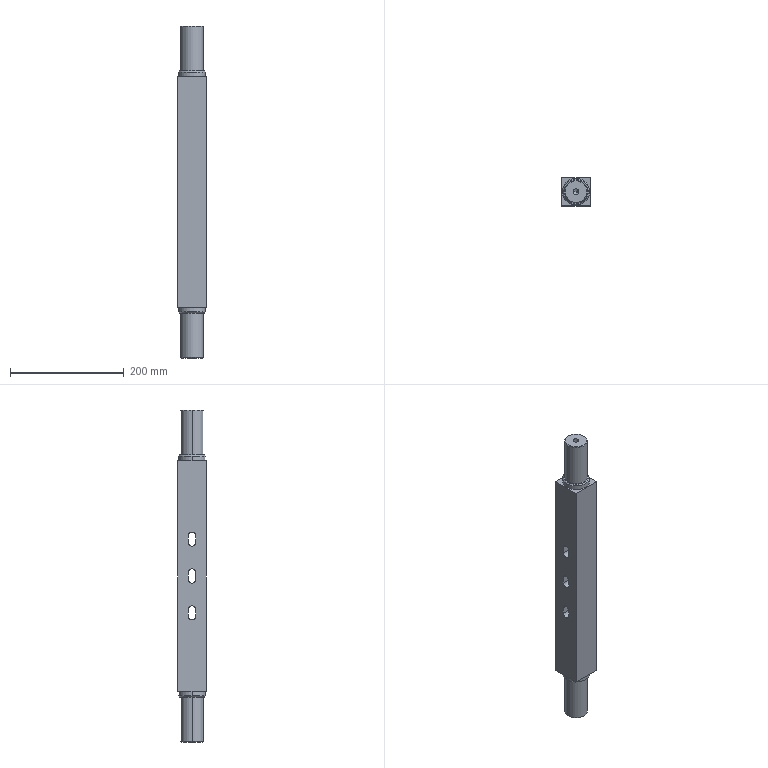Part | SolidWorks | features ICE 5, Chamfer 3, HoleWzd 2, Extrusion 1 | 1 solid | 46 faces | box 50 x 50 x 584.5 mm | volume 1201279 mm3 | cylinder 18 | plane 16 | cone 12 | commonest cylinder face diameters 13 x6 10.2 x4 40 x4 47.5 x4
STEP:
#1=CARTESIAN_POINT('',(-5.1,0.,555.25));
#2=VERTEX_POINT('',#1);
#3=CARTESIAN_POINT('',(5.1,0.,555.25));
#4=VERTEX_POINT('',#3);
#5=CARTESIAN_POINT('',(0.,0.,555.25));
#6=DIRECTION('',(0.,0.,1.));
#7=DIRECTION('',(1.,0.,0.));
#8=AXIS2_PLACEMENT_3D('',#5,#6,#7);
#9=CIRCLE('',#8,5.1);
#10=EDGE_CURVE('',#2,#4,#9,.T.);
#11=ORIENTED_EDGE('',*,*,#10,.F.);
#12=CARTESIAN_POINT('',(-5.1,0.,584.5));
#13=VERTEX_POINT('',#12);
#14=CARTESIAN_POINT('',(-5.1,0.,584.5));
#15=DIRECTION('',(0.,0.,1.));
#16=VECTOR('',#15,1000.);
#17=LINE('',#14,#16);
#18=EDGE_CURVE('',#2,#13,#17,.T.);
#19=ORIENTED_EDGE('',*,*,#18,.T.);
#20=CARTESIAN_POINT('',(5.1,0.,584.5));
#21=VERTEX_POINT('',#20);
#22=CARTESIAN_POINT('',(0.,0.,584.5));
#23=DIRECTION('',(0.,0.,1.));
#24=DIRECTION('',(1.,0.,0.));
#25=AXIS2_PLACEMENT_3D('',#22,#23,#24);
#26=CIRCLE('',#25,5.1);
#27=EDGE_CURVE('',#13,#21,#26,.T.);
#28=ORIENTED_EDGE('',*,*,#27,.T.);
#29=CARTESIAN_POINT('',(5.1,0.,584.5));
#30=DIRECTION('',(0.,0.,1.));
#31=VECTOR('',#30,1000.);
#32=LINE('',#29,#31);
#33=EDGE_CURVE('',#4,#21,#32,.T.);
#34=ORIENTED_EDGE('',*,*,#33,.F.);
#35=EDGE_LOOP('',(#11,#19,#28,#34));
#36=FACE_OUTER_BOUND('',#35,.T.);
#37=CARTESIAN_POINT('',(0.,0.,584.5));
#38=DIRECTION('',(0.,0.,1.));
#39=DIRECTION('',(1.,0.,0.));
#40=AXIS2_PLACEMENT_3D('',#37,#38,#39);
#41=CYLINDRICAL_SURFACE('',#40,5.1);
#42=ADVANCED_FACE('',(#36),#41,.F.);
#43=CARTESIAN_POINT('',(0.,0.,552.186));
#44=VERTEX_POINT('',#43);
#45=CARTESIAN_POINT('',(5.1,0.,555.25));
#46=DIRECTION('',(0.8572,0.,0.515));
#47=VECTOR('',#46,1000.);
#48=LINE('',#45,#47);
#49=EDGE_CURVE('',#44,#4,#48,.T.);
#50=ORIENTED_EDGE('',*,*,#49,.F.);
#51=CARTESIAN_POINT('',(-5.1,0.,555.25));
#52=DIRECTION('',(-0.8572,0.,0.515));
#53=VECTOR('',#52,1000.);
#54=LINE('',#51,#53);
#55=EDGE_CURVE('',#44,#2,#54,.T.);
#56=ORIENTED_EDGE('',*,*,#55,.T.);
#57=ORIENTED_EDGE('',*,*,#10,.T.);
#58=EDGE_LOOP('',(#50,#56,#57));
#59=FACE_OUTER_BOUND('',#58,.T.);
#60=CARTESIAN_POINT('',(0.,0.,555.25));
#61=DIRECTION('',(0.,0.,1.));
#62=DIRECTION('',(1.,0.,0.));
#63=AXIS2_PLACEMENT_3D('',#60,#61,#62);
#64=CONICAL_SURFACE('',#63,5.1,1.03);
#65=ADVANCED_FACE('',(#59),#64,.F.);
#66=CARTESIAN_POINT('',(5.1,0.,29.25));
#67=VERTEX_POINT('',#66);
#68=CARTESIAN_POINT('',(-5.1,0.,29.25));
#69=VERTEX_POINT('',#68);
#70=CARTESIAN_POINT('',(0.,0.,29.25));
#71=DIRECTION('',(0.,0.,-1.));
#72=DIRECTION('',(-1.,0.,0.));
#73=AXIS2_PLACEMENT_3D('',#70,#71,#72);
#74=CIRCLE('',#73,5.1);
#75=EDGE_CURVE('',#67,#69,#74,.T.);
#76=ORIENTED_EDGE('',*,*,#75,.F.);
#77=CARTESIAN_POINT('',(5.1,0.,0.));
#78=VERTEX_POINT('',#77);
#79=CARTESIAN_POINT('',(5.1,0.,0.));
#80=DIRECTION('',(0.,0.,-1.));
#81=VECTOR('',#80,1000.);
#82=LINE('',#79,#81);
#83=EDGE_CURVE('',#67,#78,#82,.T.);
#84=ORIENTED_EDGE('',*,*,#83,.T.);
#85=CARTESIAN_POINT('',(-5.1,0.,0.));
#86=VERTEX_POINT('',#85);
#87=CARTESIAN_POINT('',(0.,0.,0.));
#88=DIRECTION('',(0.,0.,-1.));
#89=DIRECTION('',(-1.,0.,0.));
#90=AXIS2_PLACEMENT_3D('',#87,#88,#89);
#91=CIRCLE('',#90,5.1);
#92=EDGE_CURVE('',#78,#86,#91,.T.);
#93=ORIENTED_EDGE('',*,*,#92,.T.);
#94=CARTESIAN_POINT('',(-5.1,0.,0.));
#95=DIRECTION('',(0.,0.,-1.));
#96=VECTOR('',#95,1000.);
#97=LINE('',#94,#96);
#98=EDGE_CURVE('',#69,#86,#97,.T.);
#99=ORIENTED_EDGE('',*,*,#98,.F.);
#100=EDGE_LOOP('',(#76,#84,#93,#99));
#101=FACE_OUTER_BOUND('',#100,.T.);
#102=CARTESIAN_POINT('',(0.,0.,0.));
#103=DIRECTION('',(0.,0.,-1.));
#104=DIRECTION('',(-1.,0.,0.));
#105=AXIS2_PLACEMENT_3D('',#102,#103,#104);
#106=CYLINDRICAL_SURFACE('',#105,5.1);
#107=ADVANCED_FACE('',(#101),#106,.F.);
#108=CARTESIAN_POINT('',(0.,0.,32.314));
#109=VERTEX_POINT('',#108);
#110=CARTESIAN_POINT('',(-5.1,0.,29.25));
#111=DIRECTION('',(-0.8572,0.,-0.515));
#112=VECTOR('',#111,1000.);
#113=LINE('',#110,#112);
#114=EDGE_CURVE('',#109,#69,#113,.T.);
#115=ORIENTED_EDGE('',*,*,#114,.F.);
#116=CARTESIAN_POINT('',(5.1,0.,29.25));
#117=DIRECTION('',(0.8572,0.,-0.515));
#118=VECTOR('',#117,1000.);
#119=LINE('',#116,#118);
#120=EDGE_CURVE('',#109,#67,#119,.T.);
#121=ORIENTED_EDGE('',*,*,#120,.T.);
#122=ORIENTED_EDGE('',*,*,#75,.T.);
#123=EDGE_LOOP('',(#115,#121,#122));
#124=FACE_OUTER_BOUND('',#123,.T.);
#125=CARTESIAN_POINT('',(0.,0.,29.25));
#126=DIRECTION('',(0.,0.,-1.));
#127=DIRECTION('',(-1.,0.,0.));
#128=AXIS2_PLACEMENT_3D('',#125,#126,#127);
#129=CONICAL_SURFACE('',#128,5.1,1.03);
#130=ADVANCED_FACE('',(#124),#129,.F.);
#131=CARTESIAN_POINT('',(19.,0.,584.5));
#132=VERTEX_POINT('',#131);
#133=CARTESIAN_POINT('',(-19.,0.,584.5));
#134=VERTEX_POINT('',#133);
#135=CARTESIAN_POINT('',(0.,0.,584.5));
#136=DIRECTION('',(0.,0.,1.));
#137=DIRECTION('',(1.,0.,0.));
#138=AXIS2_PLACEMENT_3D('',#135,#136,#137);
#139=CIRCLE('',#138,19.);
#140=EDGE_CURVE('',#132,#134,#139,.T.);
#141=ORIENTED_EDGE('',*,*,#140,.F.);
#142=CARTESIAN_POINT('',(20.,0.,583.5));
#143=VERTEX_POINT('',#142);
#144=CARTESIAN_POINT('',(19.,0.,584.5));
#145=DIRECTION('',(0.7071,0.,-0.7071));
#146=VECTOR('',#145,1000.);
#147=LINE('',#144,#146);
#148=EDGE_CURVE('',#132,#143,#147,.T.);
#149=ORIENTED_EDGE('',*,*,#148,.T.);
#150=CARTESIAN_POINT('',(-20.,0.,583.5));
#151=VERTEX_POINT('',#150);
#152=CARTESIAN_POINT('',(0.,0.,583.5));
#153=DIRECTION('',(0.,0.,-1.));
#154=DIRECTION('',(1.,0.,0.));
#155=AXIS2_PLACEMENT_3D('',#152,#153,#154);
#156=CIRCLE('',#155,20.);
#157=EDGE_CURVE('',#151,#143,#156,.T.);
#158=ORIENTED_EDGE('',*,*,#157,.F.);
#159=CARTESIAN_POINT('',(-19.,0.,584.5));
#160=DIRECTION('',(-0.7071,0.,-0.7071));
#161=VECTOR('',#160,1000.);
#162=LINE('',#159,#161);
#163=EDGE_CURVE('',#134,#151,#162,.T.);
#164=ORIENTED_EDGE('',*,*,#163,.F.);
#165=EDGE_LOOP('',(#141,#149,#158,#164));
#166=FACE_OUTER_BOUND('',#165,.T.);
#167=CARTESIAN_POINT('',(0.,0.,584.5));
#168=DIRECTION('',(0.,0.,-1.));
#169=DIRECTION('',(-1.,0.,0.));
#170=AXIS2_PLACEMENT_3D('',#167,#168,#169);
#171=CONICAL_SURFACE('',#170,19.,0.7854);
#172=ADVANCED_FACE('',(#166),#171,.T.);
#173=CARTESIAN_POINT('',(-19.,0.,0.));
#174=VERTEX_POINT('',#173);
#175=CARTESIAN_POINT('',(19.,0.,0.));
#176=VERTEX_POINT('',#175);
#177=CARTESIAN_POINT('',(0.,0.,0.));
#178=DIRECTION('',(0.,0.,-1.));
#179=DIRECTION('',(1.,0.,0.));
#180=AXIS2_PLACEMENT_3D('',#177,#178,#179);
#181=CIRCLE('',#180,19.);
#182=EDGE_CURVE('',#174,#176,#181,.T.);
#183=ORIENTED_EDGE('',*,*,#182,.F.);
#184=CARTESIAN_POINT('',(-20.,0.,1.));
#185=VERTEX_POINT('',#184);
#186=CARTESIAN_POINT('',(-20.,0.,1.));
#187=DIRECTION('',(-0.7071,0.,0.7071));
#188=VECTOR('',#187,1000.);
#189=LINE('',#186,#188);
#190=EDGE_CURVE('',#174,#185,#189,.T.);
#191=ORIENTED_EDGE('',*,*,#190,.T.);
#192=CARTESIAN_POINT('',(20.,0.,1.));
#193=VERTEX_POINT('',#192);
#194=CARTESIAN_POINT('',(0.,0.,1.));
#195=DIRECTION('',(0.,0.,1.));
#196=DIRECTION('',(1.,0.,0.));
#197=AXIS2_PLACEMENT_3D('',#194,#195,#196);
#198=CIRCLE('',#197,20.);
#199=EDGE_CURVE('',#193,#185,#198,.T.);
#200=ORIENTED_EDGE('',*,*,#199,.F.);
#201=CARTESIAN_POINT('',(20.,0.,1.));
#202=DIRECTION('',(0.7071,0.,0.7071));
#203=VECTOR('',#202,1000.);
#204=LINE('',#201,#203);
#205=EDGE_CURVE('',#176,#193,#204,.T.);
#206=ORIENTED_EDGE('',*,*,#205,.F.);
#207=EDGE_LOOP('',(#183,#191,#200,#206));
#208=FACE_OUTER_BOUND('',#207,.T.);
#209=CARTESIAN_POINT('',(0.,0.,1.));
#210=DIRECTION('',(0.,0.,1.));
#211=DIRECTION('',(1.,0.,0.));
#212=AXIS2_PLACEMENT_3D('',#209,#210,#211);
#213=CONICAL_SURFACE('',#212,20.,0.7854);
#214=ADVANCED_FACE('',(#208),#213,.T.);
#215=ORIENTED_EDGE('',*,*,#157,.T.);
#216=CARTESIAN_POINT('',(20.,0.,505.5));
#217=VERTEX_POINT('',#216);
#218=CARTESIAN_POINT('',(20.,0.,584.5));
#219=DIRECTION('',(0.,0.,-1.));
#220=VECTOR('',#219,1000.);
#221=LINE('',#218,#220);
#222=EDGE_CURVE('',#143,#217,#221,.T.);
#223=ORIENTED_EDGE('',*,*,#222,.T.);
#224=CARTESIAN_POINT('',(-20.,0.,505.5));
#225=VERTEX_POINT('',#224);
#226=CARTESIAN_POINT('',(0.,0.,505.5));
#227=DIRECTION('',(0.,0.,1.));
#228=DIRECTION('',(1.,0.,0.));
#229=AXIS2_PLACEMENT_3D('',#226,#227,#228);
#230=CIRCLE('',#229,20.);
#231=EDGE_CURVE('',#217,#225,#230,.T.);
#232=ORIENTED_EDGE('',*,*,#231,.T.);
#233=CARTESIAN_POINT('',(-20.,0.,584.5));
#234=DIRECTION('',(0.,0.,-1.));
#235=VECTOR('',#234,1000.);
#236=LINE('',#233,#235);
#237=EDGE_CURVE('',#151,#225,#236,.T.);
#238=ORIENTED_EDGE('',*,*,#237,.F.);
#239=EDGE_LOOP('',(#215,#223,#232,#238));
#240=FACE_OUTER_BOUND('',#239,.T.);
#241=CARTESIAN_POINT('',(0.,0.,584.5));
#242=DIRECTION('',(0.,0.,-1.));
#243=DIRECTION('',(-1.,0.,0.));
#244=AXIS2_PLACEMENT_3D('',#241,#242,#243);
#245=CYLINDRICAL_SURFACE('',#244,20.);
#246=ADVANCED_FACE('',(#240),#245,.T.);
#247=CARTESIAN_POINT('',(21.75,0.,505.5));
#248=VERTEX_POINT('',#247);
#249=CARTESIAN_POINT('',(-21.75,0.,505.5));
#250=VERTEX_POINT('',#249);
#251=CARTESIAN_POINT('',(0.,0.,505.5));
#252=DIRECTION('',(0.,0.,1.));
#253=DIRECTION('',(1.,0.,0.));
#254=AXIS2_PLACEMENT_3D('',#251,#252,#253);
#255=CIRCLE('',#254,21.75);
#256=EDGE_CURVE('',#248,#250,#255,.T.);
#257=ORIENTED_EDGE('',*,*,#256,.F.);
#258=CARTESIAN_POINT('',(23.75,0.,503.5));
#259=VERTEX_POINT('',#258);
#260=CARTESIAN_POINT('',(21.75,0.,505.5));
#261=DIRECTION('',(0.7071,0.,-0.7071));
#262=VECTOR('',#261,1000.);
#263=LINE('',#260,#262);
#264=EDGE_CURVE('',#248,#259,#263,.T.);
#265=ORIENTED_EDGE('',*,*,#264,.T.);
#266=CARTESIAN_POINT('',(-23.75,0.,503.5));
#267=VERTEX_POINT('',#266);
#268=CARTESIAN_POINT('',(0.,0.,503.5));
#269=DIRECTION('',(0.,0.,-1.));
#270=DIRECTION('',(1.,0.,0.));
#271=AXIS2_PLACEMENT_3D('',#268,#269,#270);
#272=CIRCLE('',#271,23.75);
#273=EDGE_CURVE('',#267,#259,#272,.T.);
#274=ORIENTED_EDGE('',*,*,#273,.F.);
#275=CARTESIAN_POINT('',(-21.75,0.,505.5));
#276=DIRECTION('',(-0.7071,0.,-0.7071));
#277=VECTOR('',#276,1000.);
#278=LINE('',#275,#277);
#279=EDGE_CURVE('',#250,#267,#278,.T.);
#280=ORIENTED_EDGE('',*,*,#279,.F.);
#281=EDGE_LOOP('',(#257,#265,#274,#280));
#282=FACE_OUTER_BOUND('',#281,.T.);
#283=CARTESIAN_POINT('',(0.,0.,505.5));
#284=DIRECTION('',(0.,0.,-1.));
#285=DIRECTION('',(-1.,0.,0.));
#286=AXIS2_PLACEMENT_3D('',#283,#284,#285);
#287=CONICAL_SURFACE('',#286,21.75,0.7854);
#288=ADVANCED_FACE('',(#282),#287,.T.);
#289=ORIENTED_EDGE('',*,*,#273,.T.);
#290=CARTESIAN_POINT('',(23.75,0.,495.5));
#291=VERTEX_POINT('',#290);
#292=CARTESIAN_POINT('',(23.75,0.,505.5));
#293=DIRECTION('',(0.,0.,-1.));
#294=VECTOR('',#293,1000.);
#295=LINE('',#292,#294);
#296=EDGE_CURVE('',#259,#291,#295,.T.);
#297=ORIENTED_EDGE('',*,*,#296,.T.);
#298=CARTESIAN_POINT('',(-23.75,0.,495.5));
#299=VERTEX_POINT('',#298);
#300=CARTESIAN_POINT('',(0.,0.,495.5));
#301=DIRECTION('',(0.,0.,1.));
#302=DIRECTION('',(1.,0.,0.));
#303=AXIS2_PLACEMENT_3D('',#300,#301,#302);
#304=CIRCLE('',#303,23.75);
#305=EDGE_CURVE('',#291,#299,#304,.T.);
#306=ORIENTED_EDGE('',*,*,#305,.T.);
#307=CARTESIAN_POINT('',(-23.75,0.,505.5));
#308=DIRECTION('',(0.,0.,-1.));
#309=VECTOR('',#308,1000.);
#310=LINE('',#307,#309);
#311=EDGE_CURVE('',#267,#299,#310,.T.);
#312=ORIENTED_EDGE('',*,*,#311,.F.);
#313=EDGE_LOOP('',(#289,#297,#306,#312));
#314=FACE_OUTER_BOUND('',#313,.T.);
#315=CARTESIAN_POINT('',(0.,0.,505.5));
#316=DIRECTION('',(0.,0.,-1.));
#317=DIRECTION('',(-1.,0.,0.));
#318=AXIS2_PLACEMENT_3D('',#315,#316,#317);
#319=CYLINDRICAL_SURFACE('',#318,23.75);
#320=ADVANCED_FACE('',(#314),#319,.T.);
#321=CARTESIAN_POINT('',(-21.75,0.,79.));
#322=VERTEX_POINT('',#321);
#323=CARTESIAN_POINT('',(21.75,0.,79.));
#324=VERTEX_POINT('',#323);
#325=CARTESIAN_POINT('',(0.,0.,79.));
#326=DIRECTION('',(0.,0.,-1.));
#327=DIRECTION('',(1.,0.,0.));
#328=AXIS2_PLACEMENT_3D('',#325,#326,#327);
#329=CIRCLE('',#328,21.75);
#330=EDGE_CURVE('',#322,#324,#329,.T.);
#331=ORIENTED_EDGE('',*,*,#330,.F.);
#332=CARTESIAN_POINT('',(-23.75,0.,81.));
#333=VERTEX_POINT('',#332);
#334=CARTESIAN_POINT('',(-23.75,0.,81.));
#335=DIRECTION('',(-0.7071,0.,0.7071));
#336=VECTOR('',#335,1000.);
#337=LINE('',#334,#336);
#338=EDGE_CURVE('',#322,#333,#337,.T.);
#339=ORIENTED_EDGE('',*,*,#338,.T.);
#340=CARTESIAN_POINT('',(23.75,0.,81.));
#341=VERTEX_POINT('',#340);
#342=CARTESIAN_POINT('',(0.,0.,81.));
#343=DIRECTION('',(0.,0.,1.));
#344=DIRECTION('',(1.,0.,0.));
#345=AXIS2_PLACEMENT_3D('',#342,#343,#344);
#346=CIRCLE('',#345,23.75);
#347=EDGE_CURVE('',#341,#333,#346,.T.);
#348=ORIENTED_EDGE('',*,*,#347,.F.);
#349=CARTESIAN_POINT('',(23.75,0.,81.));
#350=DIRECTION('',(0.7071,0.,0.7071));
#351=VECTOR('',#350,1000.);
#352=LINE('',#349,#351);
#353=EDGE_CURVE('',#324,#341,#352,.T.);
#354=ORIENTED_EDGE('',*,*,#353,.F.);
#355=EDGE_LOOP('',(#331,#339,#348,#354));
#356=FACE_OUTER_BOUND('',#355,.T.);
#357=CARTESIAN_POINT('',(0.,0.,81.));
#358=DIRECTION('',(0.,0.,1.));
#359=DIRECTION('',(1.,0.,0.));
#360=AXIS2_PLACEMENT_3D('',#357,#358,#359);
#361=CONICAL_SURFACE('',#360,23.75,0.7854);
#362=ADVANCED_FACE('',(#356),#361,.T.);
#363=CARTESIAN_POINT('',(23.75,0.,89.));
#364=VERTEX_POINT('',#363);
#365=CARTESIAN_POINT('',(-23.75,0.,89.));
#366=VERTEX_POINT('',#365);
#367=CARTESIAN_POINT('',(0.,0.,89.));
#368=DIRECTION('',(0.,0.,1.));
#369=DIRECTION('',(1.,0.,0.));
#370=AXIS2_PLACEMENT_3D('',#367,#368,#369);
#371=CIRCLE('',#370,23.75);
#372=EDGE_CURVE('',#364,#366,#371,.T.);
#373=ORIENTED_EDGE('',*,*,#372,.F.);
#374=CARTESIAN_POINT('',(23.75,0.,89.));
#375=DIRECTION('',(0.,0.,-1.));
#376=VECTOR('',#375,1000.);
#377=LINE('',#374,#376);
#378=EDGE_CURVE('',#364,#341,#377,.T.);
#379=ORIENTED_EDGE('',*,*,#378,.T.);
#380=ORIENTED_EDGE('',*,*,#347,.T.);
#381=CARTESIAN_POINT('',(-23.75,0.,89.));
#382=DIRECTION('',(0.,0.,-1.));
#383=VECTOR('',#382,1000.);
#384=LINE('',#381,#383);
#385=EDGE_CURVE('',#366,#333,#384,.T.);
#386=ORIENTED_EDGE('',*,*,#385,.F.);
#387=EDGE_LOOP('',(#373,#379,#380,#386));
#388=FACE_OUTER_BOUND('',#387,.T.);
#389=CARTESIAN_POINT('',(0.,0.,89.));
#390=DIRECTION('',(0.,0.,-1.));
#391=DIRECTION('',(-1.,0.,0.));
#392=AXIS2_PLACEMENT_3D('',#389,#390,#391);
#393=CYLINDRICAL_SURFACE('',#392,23.75);
#394=ADVANCED_FACE('',(#388),#393,.T.);
#395=CARTESIAN_POINT('',(20.,0.,79.));
#396=VERTEX_POINT('',#395);
#397=CARTESIAN_POINT('',(-20.,0.,79.));
#398=VERTEX_POINT('',#397);
#399=CARTESIAN_POINT('',(0.,0.,79.));
#400=DIRECTION('',(0.,0.,1.));
#401=DIRECTION('',(1.,0.,0.));
#402=AXIS2_PLACEMENT_3D('',#399,#400,#401);
#403=CIRCLE('',#402,20.);
#404=EDGE_CURVE('',#396,#398,#403,.T.);
#405=ORIENTED_EDGE('',*,*,#404,.F.);
#406=CARTESIAN_POINT('',(20.,0.,79.));
#407=DIRECTION('',(0.,0.,-1.));
#408=VECTOR('',#407,1000.);
#409=LINE('',#406,#408);
#410=EDGE_CURVE('',#396,#193,#409,.T.);
#411=ORIENTED_EDGE('',*,*,#410,.T.);
#412=ORIENTED_EDGE('',*,*,#199,.T.);
#413=CARTESIAN_POINT('',(-20.,0.,79.));
#414=DIRECTION('',(0.,0.,-1.));
#415=VECTOR('',#414,1000.);
#416=LINE('',#413,#415);
#417=EDGE_CURVE('',#398,#185,#416,.T.);
#418=ORIENTED_EDGE('',*,*,#417,.F.);
#419=EDGE_LOOP('',(#405,#411,#412,#418));
#420=FACE_OUTER_BOUND('',#419,.T.);
#421=CARTESIAN_POINT('',(0.,0.,79.));
#422=DIRECTION('',(0.,0.,-1.));
#423=DIRECTION('',(-1.,0.,0.));
#424=AXIS2_PLACEMENT_3D('',#421,#422,#423);
#425=CYLINDRICAL_SURFACE('',#424,20.);
#426=ADVANCED_FACE('',(#420),#425,.T.);
#427=ORIENTED_EDGE('',*,*,#410,.F.);
#428=CARTESIAN_POINT('',(0.,0.,79.));
#429=DIRECTION('',(0.,0.,1.));
#430=DIRECTION('',(1.,0.,0.));
#431=AXIS2_PLACEMENT_3D('',#428,#429,#430);
#432=CIRCLE('',#431,20.);
#433=EDGE_CURVE('',#398,#396,#432,.T.);
#434=ORIENTED_EDGE('',*,*,#433,.F.);
#435=ORIENTED_EDGE('',*,*,#417,.T.);
#436=CARTESIAN_POINT('',(0.,0.,1.));
#437=DIRECTION('',(0.,0.,1.));
#438=DIRECTION('',(1.,0.,0.));
#439=AXIS2_PLACEMENT_3D('',#436,#437,#438);
#440=CIRCLE('',#439,20.);
#441=EDGE_CURVE('',#185,#193,#440,.T.);
#442=ORIENTED_EDGE('',*,*,#441,.T.);
#443=EDGE_LOOP('',(#427,#434,#435,#442));
#444=FACE_OUTER_BOUND('',#443,.T.);
#445=CARTESIAN_POINT('',(0.,0.,79.));
#446=DIRECTION('',(0.,0.,-1.));
#447=DIRECTION('',(-1.,0.,0.));
#448=AXIS2_PLACEMENT_3D('',#445,#446,#447);
#449=CYLINDRICAL_SURFACE('',#448,20.);
#450=ADVANCED_FACE('',(#444),#449,.T.);
#451=CARTESIAN_POINT('',(0.,0.,0.));
#452=DIRECTION('',(0.,0.,-1.));
#453=DIRECTION('',(-1.,0.,0.));
#454=AXIS2_PLACEMENT_3D('',#451,#452,#453);
#455=CIRCLE('',#454,5.1);
#456=EDGE_CURVE('',#86,#78,#455,.T.);
#457=ORIENTED_EDGE('',*,*,#456,.F.);
#458=ORIENTED_EDGE('',*,*,#92,.F.);
#459=EDGE_LOOP('',(#457,#458));
#460=FACE_BOUND('',#459,.T.);
#461=CARTESIAN_POINT('',(0.,0.,0.));
#462=DIRECTION('',(0.,0.,-1.));
#463=DIRECTION('',(1.,0.,0.));
#464=AXIS2_PLACEMENT_3D('',#461,#462,#463);
#465=CIRCLE('',#464,19.);
#466=EDGE_CURVE('',#176,#174,#465,.T.);
#467=ORIENTED_EDGE('',*,*,#466,.T.);
#468=ORIENTED_EDGE('',*,*,#182,.T.);
#469=EDGE_LOOP('',(#467,#468));
#470=FACE_OUTER_BOUND('',#469,.T.);
#471=CARTESIAN_POINT('',(0.,0.,0.));
#472=DIRECTION('',(0.,0.,1.));
#473=DIRECTION('',(1.,0.,0.));
#474=AXIS2_PLACEMENT_3D('',#471,#472,#473);
#475=PLANE('',#474);
#476=ADVANCED_FACE('',(#460,#470),#475,.F.);
#477=ORIENTED_EDGE('',*,*,#378,.F.);
#478=CARTESIAN_POINT('',(0.,0.,89.));
#479=DIRECTION('',(0.,0.,1.));
#480=DIRECTION('',(1.,0.,0.));
#481=AXIS2_PLACEMENT_3D('',#478,#479,#480);
#482=CIRCLE('',#481,23.75);
#483=EDGE_CURVE('',#366,#364,#482,.T.);
#484=ORIENTED_EDGE('',*,*,#483,.F.);
#485=ORIENTED_EDGE('',*,*,#385,.T.);
#486=CARTESIAN_POINT('',(0.,0.,81.));
#487=DIRECTION('',(0.,0.,1.));
#488=DIRECTION('',(1.,0.,0.));
#489=AXIS2_PLACEMENT_3D('',#486,#487,#488);
#490=CIRCLE('',#489,23.75);
#491=EDGE_CURVE('',#333,#341,#490,.T.);
#492=ORIENTED_EDGE('',*,*,#491,.T.);
#493=EDGE_LOOP('',(#477,#484,#485,#492));
#494=FACE_OUTER_BOUND('',#493,.T.);
#495=CARTESIAN_POINT('',(0.,0.,89.));
#496=DIRECTION('',(0.,0.,-1.));
#497=DIRECTION('',(-1.,0.,0.));
#498=AXIS2_PLACEMENT_3D('',#495,#496,#497);
#499=CYLINDRICAL_SURFACE('',#498,23.75);
#500=ADVANCED_FACE('',(#494),#499,.T.);
#501=CARTESIAN_POINT('',(0.,0.,79.));
#502=DIRECTION('',(0.,0.,-1.));
#503=DIRECTION('',(1.,0.,0.));
#504=AXIS2_PLACEMENT_3D('',#501,#502,#503);
#505=CIRCLE('',#504,21.75);
#506=EDGE_CURVE('',#324,#322,#505,.T.);
#507=ORIENTED_EDGE('',*,*,#506,.T.);
#508=ORIENTED_EDGE('',*,*,#330,.T.);
#509=EDGE_LOOP('',(#507,#508));
#510=FACE_OUTER_BOUND('',#509,.T.);
#511=ORIENTED_EDGE('',*,*,#433,.T.);
#512=ORIENTED_EDGE('',*,*,#404,.T.);
#513=EDGE_LOOP('',(#511,#512));
#514=FACE_BOUND('',#513,.T.);
#515=CARTESIAN_POINT('',(0.,0.,79.));
#516=DIRECTION('',(0.,0.,1.));
#517=DIRECTION('',(1.,0.,0.));
#518=AXIS2_PLACEMENT_3D('',#515,#516,#517);
#519=PLANE('',#518);
#520=ADVANCED_FACE('',(#510,#514),#519,.F.);
#521=ORIENTED_EDGE('',*,*,#338,.F.);
#522=ORIENTED_EDGE('',*,*,#506,.F.);
#523=ORIENTED_EDGE('',*,*,#353,.T.);
#524=ORIENTED_EDGE('',*,*,#491,.F.);
#525=EDGE_LOOP('',(#521,#522,#523,#524));
#526=FACE_OUTER_BOUND('',#525,.T.);
#527=CARTESIAN_POINT('',(0.,0.,81.));
#528=DIRECTION('',(0.,0.,1.));
#529=DIRECTION('',(1.,0.,0.));
#530=AXIS2_PLACEMENT_3D('',#527,#528,#529);
#531=CONICAL_SURFACE('',#530,23.75,0.7854);
#532=ADVANCED_FACE('',(#526),#531,.T.);
#533=CARTESIAN_POINT('',(-25.,6.5,351.25));
#534=VERTEX_POINT('',#533);
#535=CARTESIAN_POINT('',(-25.,6.5,363.25));
#536=VERTEX_POINT('',#535);
#537=CARTESIAN_POINT('',(-25.,6.5,495.5));
#538=DIRECTION('',(0.,0.,1.));
#539=VECTOR('',#538,1000.);
#540=LINE('',#537,#539);
#541=EDGE_CURVE('',#534,#536,#540,.T.);
#542=ORIENTED_EDGE('',*,*,#541,.T.);
#543=CARTESIAN_POINT('',(-25.,-6.5,363.25));
#544=VERTEX_POINT('',#543);
#545=CARTESIAN_POINT('',(-25.,0.,363.25));
#546=DIRECTION('',(1.,0.,0.));
#547=DIRECTION('',(0.,1.,0.));
#548=AXIS2_PLACEMENT_3D('',#545,#546,#547);
#549=CIRCLE('',#548,6.5);
#550=EDGE_CURVE('',#536,#544,#549,.T.);
#551=ORIENTED_EDGE('',*,*,#550,.T.);
#552=CARTESIAN_POINT('',(-25.,-6.5,351.25));
#553=VERTEX_POINT('',#552);
#554=CARTESIAN_POINT('',(-25.,-6.5,495.5));
#555=DIRECTION('',(0.,0.,-1.));
#556=VECTOR('',#555,1000.);
#557=LINE('',#554,#556);
#558=EDGE_CURVE('',#544,#553,#557,.T.);
#559=ORIENTED_EDGE('',*,*,#558,.T.);
#560=CARTESIAN_POINT('',(-25.,0.,351.25));
#561=DIRECTION('',(1.,0.,0.));
#562=DIRECTION('',(0.,1.,0.));
#563=AXIS2_PLACEMENT_3D('',#560,#561,#562);
#564=CIRCLE('',#563,6.5);
#565=EDGE_CURVE('',#553,#534,#564,.T.);
#566=ORIENTED_EDGE('',*,*,#565,.T.);
#567=EDGE_LOOP('',(#542,#551,#559,#566));
#568=FACE_BOUND('',#567,.T.);
#569=CARTESIAN_POINT('',(-25.,6.5,286.25));
#570=VERTEX_POINT('',#569);
#571=CARTESIAN_POINT('',(-25.,6.5,298.25));
#572=VERTEX_POINT('',#571);
#573=CARTESIAN_POINT('',(-25.,6.5,495.5));
#574=DIRECTION('',(0.,0.,1.));
#575=VECTOR('',#574,1000.);
#576=LINE('',#573,#575);
#577=EDGE_CURVE('',#570,#572,#576,.T.);
#578=ORIENTED_EDGE('',*,*,#577,.T.);
#579=CARTESIAN_POINT('',(-25.,-6.5,298.25));
#580=VERTEX_POINT('',#579);
#581=CARTESIAN_POINT('',(-25.,0.,298.25));
#582=DIRECTION('',(1.,0.,0.));
#583=DIRECTION('',(0.,1.,0.));
#584=AXIS2_PLACEMENT_3D('',#581,#582,#583);
#585=CIRCLE('',#584,6.5);
#586=EDGE_CURVE('',#572,#580,#585,.T.);
#587=ORIENTED_EDGE('',*,*,#586,.T.);
#588=CARTESIAN_POINT('',(-25.,-6.5,286.25));
#589=VERTEX_POINT('',#588);
#590=CARTESIAN_POINT('',(-25.,-6.5,495.5));
#591=DIRECTION('',(0.,0.,-1.));
#592=VECTOR('',#591,1000.);
#593=LINE('',#590,#592);
#594=EDGE_CURVE('',#580,#589,#593,.T.);
#595=ORIENTED_EDGE('',*,*,#594,.T.);
#596=CARTESIAN_POINT('',(-25.,0.,286.25));
#597=DIRECTION('',(1.,0.,0.));
#598=DIRECTION('',(0.,1.,0.));
#599=AXIS2_PLACEMENT_3D('',#596,#597,#598);
#600=CIRCLE('',#599,6.5);
#601=EDGE_CURVE('',#589,#570,#600,.T.);
#602=ORIENTED_EDGE('',*,*,#601,.T.);
#603=EDGE_LOOP('',(#578,#587,#595,#602));
#604=FACE_BOUND('',#603,.T.);
#605=CARTESIAN_POINT('',(-25.,6.5,221.25));
#606=VERTEX_POINT('',#605);
#607=CARTESIAN_POINT('',(-25.,6.5,233.25));
#608=VERTEX_POINT('',#607);
#609=CARTESIAN_POINT('',(-25.,6.5,495.5));
#610=DIRECTION('',(0.,0.,1.));
#611=VECTOR('',#610,1000.);
#612=LINE('',#609,#611);
#613=EDGE_CURVE('',#606,#608,#612,.T.);
#614=ORIENTED_EDGE('',*,*,#613,.T.);
#615=CARTESIAN_POINT('',(-25.,-6.5,233.25));
#616=VERTEX_POINT('',#615);
#617=CARTESIAN_POINT('',(-25.,0.,233.25));
#618=DIRECTION('',(1.,0.,0.));
#619=DIRECTION('',(0.,1.,0.));
#620=AXIS2_PLACEMENT_3D('',#617,#618,#619);
#621=CIRCLE('',#620,6.5);
#622=EDGE_CURVE('',#608,#616,#621,.T.);
#623=ORIENTED_EDGE('',*,*,#622,.T.);
#624=CARTESIAN_POINT('',(-25.,-6.5,221.25));
#625=VERTEX_POINT('',#624);
#626=CARTESIAN_POINT('',(-25.,-6.5,495.5));
#627=DIRECTION('',(0.,0.,-1.));
#628=VECTOR('',#627,1000.);
#629=LINE('',#626,#628);
#630=EDGE_CURVE('',#616,#625,#629,.T.);
#631=ORIENTED_EDGE('',*,*,#630,.T.);
#632=CARTESIAN_POINT('',(-25.,0.,221.25));
#633=DIRECTION('',(1.,0.,0.));
#634=DIRECTION('',(0.,1.,0.));
#635=AXIS2_PLACEMENT_3D('',#632,#633,#634);
#636=CIRCLE('',#635,6.5);
#637=EDGE_CURVE('',#625,#606,#636,.T.);
#638=ORIENTED_EDGE('',*,*,#637,.T.);
#639=EDGE_LOOP('',(#614,#623,#631,#638));
#640=FACE_BOUND('',#639,.T.);
#641=CARTESIAN_POINT('',(-25.,25.,89.));
#642=VERTEX_POINT('',#641);
#643=CARTESIAN_POINT('',(-25.,-25.,89.));
#644=VERTEX_POINT('',#643);
#645=CARTESIAN_POINT('',(-25.,25.,89.));
#646=DIRECTION('',(0.,-1.,0.));
#647=VECTOR('',#646,1000.);
#648=LINE('',#645,#647);
#649=EDGE_CURVE('',#642,#644,#648,.T.);
#650=ORIENTED_EDGE('',*,*,#649,.T.);
#651=CARTESIAN_POINT('',(-25.,-25.,495.5));
#652=VERTEX_POINT('',#651);
#653=CARTESIAN_POINT('',(-25.,-25.,495.5));
#654=DIRECTION('',(0.,0.,-1.));
#655=VECTOR('',#654,1000.);
#656=LINE('',#653,#655);
#657=EDGE_CURVE('',#652,#644,#656,.T.);
#658=ORIENTED_EDGE('',*,*,#657,.F.);
#659=CARTESIAN_POINT('',(-25.,25.,495.5));
#660=VERTEX_POINT('',#659);
#661=CARTESIAN_POINT('',(-25.,25.,495.5));
#662=DIRECTION('',(0.,-1.,0.));
#663=VECTOR('',#662,1000.);
#664=LINE('',#661,#663);
#665=EDGE_CURVE('',#660,#652,#664,.T.);
#666=ORIENTED_EDGE('',*,*,#665,.F.);
#667=CARTESIAN_POINT('',(-25.,25.,495.5));
#668=DIRECTION('',(0.,0.,-1.));
#669=VECTOR('',#668,1000.);
#670=LINE('',#667,#669);
#671=EDGE_CURVE('',#660,#642,#670,.T.);
#672=ORIENTED_EDGE('',*,*,#671,.T.);
#673=EDGE_LOOP('',(#650,#658,#666,#672));
#674=FACE_OUTER_BOUND('',#673,.T.);
#675=CARTESIAN_POINT('',(-25.,25.,495.5));
#676=DIRECTION('',(1.,0.,0.));
#677=DIRECTION('',(0.,1.,0.));
#678=AXIS2_PLACEMENT_3D('',#675,#676,#677);
#679=PLANE('',#678);
#680=ADVANCED_FACE('',(#568,#604,#640,#674),#679,.F.);
#681=CARTESIAN_POINT('',(25.,-25.,89.));
#682=VERTEX_POINT('',#681);
#683=CARTESIAN_POINT('',(25.,-25.,89.));
#684=DIRECTION('',(1.,0.,0.));
#685=VECTOR('',#684,1000.);
#686=LINE('',#683,#685);
#687=EDGE_CURVE('',#644,#682,#686,.T.);
#688=ORIENTED_EDGE('',*,*,#687,.T.);
#689=CARTESIAN_POINT('',(25.,-25.,495.5));
#690=VERTEX_POINT('',#689);
#691=CARTESIAN_POINT('',(25.,-25.,495.5));
#692=DIRECTION('',(0.,0.,-1.));
#693=VECTOR('',#692,1000.);
#694=LINE('',#691,#693);
#695=EDGE_CURVE('',#690,#682,#694,.T.);
#696=ORIENTED_EDGE('',*,*,#695,.F.);
#697=CARTESIAN_POINT('',(25.,-25.,495.5));
#698=DIRECTION('',(1.,0.,0.));
#699=VECTOR('',#698,1000.);
#700=LINE('',#697,#699);
#701=EDGE_CURVE('',#652,#690,#700,.T.);
#702=ORIENTED_EDGE('',*,*,#701,.F.);
#703=ORIENTED_EDGE('',*,*,#657,.T.);
#704=EDGE_LOOP('',(#688,#696,#702,#703));
#705=FACE_OUTER_BOUND('',#704,.T.);
#706=CARTESIAN_POINT('',(25.,-25.,495.5));
#707=DIRECTION('',(0.,1.,0.));
#708=DIRECTION('',(-1.,0.,0.));
#709=AXIS2_PLACEMENT_3D('',#706,#707,#708);
#710=PLANE('',#709);
#711=ADVANCED_FACE('',(#705),#710,.F.);
#712=CARTESIAN_POINT('',(25.,-6.5,363.25));
#713=VERTEX_POINT('',#712);
#714=CARTESIAN_POINT('',(25.,-6.5,351.25));
#715=VERTEX_POINT('',#714);
#716=CARTESIAN_POINT('',(25.,-6.5,363.25));
#717=DIRECTION('',(0.,0.,-1.));
#718=VECTOR('',#717,1000.);
#719=LINE('',#716,#718);
#720=EDGE_CURVE('',#713,#715,#719,.T.);
#721=ORIENTED_EDGE('',*,*,#720,.F.);
#722=CARTESIAN_POINT('',(25.,6.5,363.25));
#723=VERTEX_POINT('',#722);
#724=CARTESIAN_POINT('',(25.,0.,363.25));
#725=DIRECTION('',(1.,0.,0.));
#726=DIRECTION('',(0.,1.,0.));
#727=AXIS2_PLACEMENT_3D('',#724,#725,#726);
#728=CIRCLE('',#727,6.5);
#729=EDGE_CURVE('',#723,#713,#728,.T.);
#730=ORIENTED_EDGE('',*,*,#729,.F.);
#731=CARTESIAN_POINT('',(25.,6.5,351.25));
#732=VERTEX_POINT('',#731);
#733=CARTESIAN_POINT('',(25.,6.5,363.25));
#734=DIRECTION('',(0.,0.,1.));
#735=VECTOR('',#734,1000.);
#736=LINE('',#733,#735);
#737=EDGE_CURVE('',#732,#723,#736,.T.);
#738=ORIENTED_EDGE('',*,*,#737,.F.);
#739=CARTESIAN_POINT('',(25.,0.,351.25));
#740=DIRECTION('',(1.,0.,0.));
#741=DIRECTION('',(0.,1.,0.));
#742=AXIS2_PLACEMENT_3D('',#739,#740,#741);
#743=CIRCLE('',#742,6.5);
#744=EDGE_CURVE('',#715,#732,#743,.T.);
#745=ORIENTED_EDGE('',*,*,#744,.F.);
#746=EDGE_LOOP('',(#721,#730,#738,#745));
#747=FACE_BOUND('',#746,.T.);
#748=CARTESIAN_POINT('',(25.,-6.5,298.25));
#749=VERTEX_POINT('',#748);
#750=CARTESIAN_POINT('',(25.,-6.5,286.25));
#751=VERTEX_POINT('',#750);
#752=CARTESIAN_POINT('',(25.,-6.5,298.25));
#753=DIRECTION('',(0.,0.,-1.));
#754=VECTOR('',#753,1000.);
#755=LINE('',#752,#754);
#756=EDGE_CURVE('',#749,#751,#755,.T.);
#757=ORIENTED_EDGE('',*,*,#756,.F.);
#758=CARTESIAN_POINT('',(25.,6.5,298.25));
#759=VERTEX_POINT('',#758);
#760=CARTESIAN_POINT('',(25.,0.,298.25));
#761=DIRECTION('',(1.,0.,0.));
#762=DIRECTION('',(0.,1.,0.));
#763=AXIS2_PLACEMENT_3D('',#760,#761,#762);
#764=CIRCLE('',#763,6.5);
#765=EDGE_CURVE('',#759,#749,#764,.T.);
#766=ORIENTED_EDGE('',*,*,#765,.F.);
#767=CARTESIAN_POINT('',(25.,6.5,286.25));
#768=VERTEX_POINT('',#767);
#769=CARTESIAN_POINT('',(25.,6.5,298.25));
#770=DIRECTION('',(0.,0.,1.));
#771=VECTOR('',#770,1000.);
#772=LINE('',#769,#771);
#773=EDGE_CURVE('',#768,#759,#772,.T.);
#774=ORIENTED_EDGE('',*,*,#773,.F.);
#775=CARTESIAN_POINT('',(25.,0.,286.25));
#776=DIRECTION('',(1.,0.,0.));
#777=DIRECTION('',(0.,1.,0.));
#778=AXIS2_PLACEMENT_3D('',#775,#776,#777);
#779=CIRCLE('',#778,6.5);
#780=EDGE_CURVE('',#751,#768,#779,.T.);
#781=ORIENTED_EDGE('',*,*,#780,.F.);
#782=EDGE_LOOP('',(#757,#766,#774,#781));
#783=FACE_BOUND('',#782,.T.);
#784=CARTESIAN_POINT('',(25.,-6.5,233.25));
#785=VERTEX_POINT('',#784);
#786=CARTESIAN_POINT('',(25.,-6.5,221.25));
#787=VERTEX_POINT('',#786);
#788=CARTESIAN_POINT('',(25.,-6.5,233.25));
#789=DIRECTION('',(0.,0.,-1.));
#790=VECTOR('',#789,1000.);
#791=LINE('',#788,#790);
#792=EDGE_CURVE('',#785,#787,#791,.T.);
#793=ORIENTED_EDGE('',*,*,#792,.F.);
#794=CARTESIAN_POINT('',(25.,6.5,233.25));
#795=VERTEX_POINT('',#794);
#796=CARTESIAN_POINT('',(25.,0.,233.25));
#797=DIRECTION('',(1.,0.,0.));
#798=DIRECTION('',(0.,1.,0.));
#799=AXIS2_PLACEMENT_3D('',#796,#797,#798);
#800=CIRCLE('',#799,6.5);
#801=EDGE_CURVE('',#795,#785,#800,.T.);
#802=ORIENTED_EDGE('',*,*,#801,.F.);
#803=CARTESIAN_POINT('',(25.,6.5,221.25));
#804=VERTEX_POINT('',#803);
#805=CARTESIAN_POINT('',(25.,6.5,233.25));
#806=DIRECTION('',(0.,0.,1.));
#807=VECTOR('',#806,1000.);
#808=LINE('',#805,#807);
#809=EDGE_CURVE('',#804,#795,#808,.T.);
#810=ORIENTED_EDGE('',*,*,#809,.F.);
#811=CARTESIAN_POINT('',(25.,0.,221.25));
#812=DIRECTION('',(1.,0.,0.));
#813=DIRECTION('',(0.,1.,0.));
#814=AXIS2_PLACEMENT_3D('',#811,#812,#813);
#815=CIRCLE('',#814,6.5);
#816=EDGE_CURVE('',#787,#804,#815,.T.);
#817=ORIENTED_EDGE('',*,*,#816,.F.);
#818=EDGE_LOOP('',(#793,#802,#810,#817));
#819=FACE_BOUND('',#818,.T.);
#820=CARTESIAN_POINT('',(25.,25.,89.));
#821=VERTEX_POINT('',#820);
#822=CARTESIAN_POINT('',(25.,25.,89.));
#823=DIRECTION('',(0.,1.,0.));
#824=VECTOR('',#823,1000.);
#825=LINE('',#822,#824);
#826=EDGE_CURVE('',#682,#821,#825,.T.);
#827=ORIENTED_EDGE('',*,*,#826,.T.);
#828=CARTESIAN_POINT('',(25.,25.,495.5));
#829=VERTEX_POINT('',#828);
#830=CARTESIAN_POINT('',(25.,25.,495.5));
#831=DIRECTION('',(0.,0.,-1.));
#832=VECTOR('',#831,1000.);
#833=LINE('',#830,#832);
#834=EDGE_CURVE('',#829,#821,#833,.T.);
#835=ORIENTED_EDGE('',*,*,#834,.F.);
#836=CARTESIAN_POINT('',(25.,25.,495.5));
#837=DIRECTION('',(0.,1.,0.));
#838=VECTOR('',#837,1000.);
#839=LINE('',#836,#838);
#840=EDGE_CURVE('',#690,#829,#839,.T.);
#841=ORIENTED_EDGE('',*,*,#840,.F.);
#842=ORIENTED_EDGE('',*,*,#695,.T.);
#843=EDGE_LOOP('',(#827,#835,#841,#842));
#844=FACE_OUTER_BOUND('',#843,.T.);
#845=CARTESIAN_POINT('',(25.,25.,495.5));
#846=DIRECTION('',(-1.,0.,0.));
#847=DIRECTION('',(0.,-1.,0.));
#848=AXIS2_PLACEMENT_3D('',#845,#846,#847);
#849=PLANE('',#848);
#850=ADVANCED_FACE('',(#747,#783,#819,#844),#849,.F.);
#851=CARTESIAN_POINT('',(25.,25.,89.));
#852=DIRECTION('',(-1.,0.,0.));
#853=VECTOR('',#852,1000.);
#854=LINE('',#851,#853);
#855=EDGE_CURVE('',#821,#642,#854,.T.);
#856=ORIENTED_EDGE('',*,*,#855,.T.);
#857=ORIENTED_EDGE('',*,*,#671,.F.);
#858=CARTESIAN_POINT('',(25.,25.,495.5));
#859=DIRECTION('',(-1.,0.,0.));
#860=VECTOR('',#859,1000.);
#861=LINE('',#858,#860);
#862=EDGE_CURVE('',#829,#660,#861,.T.);
#863=ORIENTED_EDGE('',*,*,#862,.F.);
#864=ORIENTED_EDGE('',*,*,#834,.T.);
#865=EDGE_LOOP('',(#856,#857,#863,#864));
#866=FACE_OUTER_BOUND('',#865,.T.);
#867=CARTESIAN_POINT('',(25.,25.,495.5));
#868=DIRECTION('',(0.,-1.,0.));
#869=DIRECTION('',(1.,0.,0.));
#870=AXIS2_PLACEMENT_3D('',#867,#868,#869);
#871=PLANE('',#870);
#872=ADVANCED_FACE('',(#866),#871,.F.);
#873=CARTESIAN_POINT('',(0.,0.,495.5));
#874=DIRECTION('',(0.,0.,1.));
#875=DIRECTION('',(1.,0.,0.));
#876=AXIS2_PLACEMENT_3D('',#873,#874,#875);
#877=CIRCLE('',#876,23.75);
#878=EDGE_CURVE('',#299,#291,#877,.T.);
#879=ORIENTED_EDGE('',*,*,#878,.F.);
#880=ORIENTED_EDGE('',*,*,#305,.F.);
#881=EDGE_LOOP('',(#879,#880));
#882=FACE_BOUND('',#881,.T.);
#883=ORIENTED_EDGE('',*,*,#665,.T.);
#884=ORIENTED_EDGE('',*,*,#701,.T.);
#885=ORIENTED_EDGE('',*,*,#840,.T.);
#886=ORIENTED_EDGE('',*,*,#862,.T.);
#887=EDGE_LOOP('',(#883,#884,#885,#886));
#888=FACE_OUTER_BOUND('',#887,.T.);
#889=CARTESIAN_POINT('',(0.,0.,495.5));
#890=DIRECTION('',(0.,0.,-1.));
#891=DIRECTION('',(-1.,0.,0.));
#892=AXIS2_PLACEMENT_3D('',#889,#890,#891);
#893=PLANE('',#892);
#894=ADVANCED_FACE('',(#882,#888),#893,.F.);
#895=ORIENTED_EDGE('',*,*,#483,.T.);
#896=ORIENTED_EDGE('',*,*,#372,.T.);
#897=EDGE_LOOP('',(#895,#896));
#898=FACE_BOUND('',#897,.T.);
#899=ORIENTED_EDGE('',*,*,#649,.F.);
#900=ORIENTED_EDGE('',*,*,#855,.F.);
#901=ORIENTED_EDGE('',*,*,#826,.F.);
#902=ORIENTED_EDGE('',*,*,#687,.F.);
#903=EDGE_LOOP('',(#899,#900,#901,#902));
#904=FACE_OUTER_BOUND('',#903,.T.);
#905=CARTESIAN_POINT('',(0.,0.,89.));
#906=DIRECTION('',(0.,0.,-1.));
#907=DIRECTION('',(-1.,0.,0.));
#908=AXIS2_PLACEMENT_3D('',#905,#906,#907);
#909=PLANE('',#908);
#910=ADVANCED_FACE('',(#898,#904),#909,.T.);
#911=ORIENTED_EDGE('',*,*,#296,.F.);
#912=CARTESIAN_POINT('',(0.,0.,503.5));
#913=DIRECTION('',(0.,0.,-1.));
#914=DIRECTION('',(1.,0.,0.));
#915=AXIS2_PLACEMENT_3D('',#912,#913,#914);
#916=CIRCLE('',#915,23.75);
#917=EDGE_CURVE('',#259,#267,#916,.T.);
#918=ORIENTED_EDGE('',*,*,#917,.T.);
#919=ORIENTED_EDGE('',*,*,#311,.T.);
#920=ORIENTED_EDGE('',*,*,#878,.T.);
#921=EDGE_LOOP('',(#911,#918,#919,#920));
#922=FACE_OUTER_BOUND('',#921,.T.);
#923=CARTESIAN_POINT('',(0.,0.,505.5));
#924=DIRECTION('',(0.,0.,-1.));
#925=DIRECTION('',(-1.,0.,0.));
#926=AXIS2_PLACEMENT_3D('',#923,#924,#925);
#927=CYLINDRICAL_SURFACE('',#926,23.75);
#928=ADVANCED_FACE('',(#922),#927,.T.);
#929=CARTESIAN_POINT('',(0.,0.,505.5));
#930=DIRECTION('',(0.,0.,1.));
#931=DIRECTION('',(1.,0.,0.));
#932=AXIS2_PLACEMENT_3D('',#929,#930,#931);
#933=CIRCLE('',#932,20.);
#934=EDGE_CURVE('',#225,#217,#933,.T.);
#935=ORIENTED_EDGE('',*,*,#934,.F.);
#936=ORIENTED_EDGE('',*,*,#231,.F.);
#937=EDGE_LOOP('',(#935,#936));
#938=FACE_BOUND('',#937,.T.);
#939=CARTESIAN_POINT('',(0.,0.,505.5));
#940=DIRECTION('',(0.,0.,1.));
#941=DIRECTION('',(1.,0.,0.));
#942=AXIS2_PLACEMENT_3D('',#939,#940,#941);
#943=CIRCLE('',#942,21.75);
#944=EDGE_CURVE('',#250,#248,#943,.T.);
#945=ORIENTED_EDGE('',*,*,#944,.T.);
#946=ORIENTED_EDGE('',*,*,#256,.T.);
#947=EDGE_LOOP('',(#945,#946));
#948=FACE_OUTER_BOUND('',#947,.T.);
#949=CARTESIAN_POINT('',(0.,0.,505.5));
#950=DIRECTION('',(0.,0.,1.));
#951=DIRECTION('',(1.,0.,0.));
#952=AXIS2_PLACEMENT_3D('',#949,#950,#951);
#953=PLANE('',#952);
#954=ADVANCED_FACE('',(#938,#948),#953,.T.);
#955=ORIENTED_EDGE('',*,*,#264,.F.);
#956=ORIENTED_EDGE('',*,*,#944,.F.);
#957=ORIENTED_EDGE('',*,*,#279,.T.);
#958=ORIENTED_EDGE('',*,*,#917,.F.);
#959=EDGE_LOOP('',(#955,#956,#957,#958));
#960=FACE_OUTER_BOUND('',#959,.T.);
#961=CARTESIAN_POINT('',(0.,0.,505.5));
#962=DIRECTION('',(0.,0.,-1.));
#963=DIRECTION('',(-1.,0.,0.));
#964=AXIS2_PLACEMENT_3D('',#961,#962,#963);
#965=CONICAL_SURFACE('',#964,21.75,0.7854);
#966=ADVANCED_FACE('',(#960),#965,.T.);
#967=ORIENTED_EDGE('',*,*,#222,.F.);
#968=CARTESIAN_POINT('',(0.,0.,583.5));
#969=DIRECTION('',(0.,0.,-1.));
#970=DIRECTION('',(1.,0.,0.));
#971=AXIS2_PLACEMENT_3D('',#968,#969,#970);
#972=CIRCLE('',#971,20.);
#973=EDGE_CURVE('',#143,#151,#972,.T.);
#974=ORIENTED_EDGE('',*,*,#973,.T.);
#975=ORIENTED_EDGE('',*,*,#237,.T.);
#976=ORIENTED_EDGE('',*,*,#934,.T.);
#977=EDGE_LOOP('',(#967,#974,#975,#976));
#978=FACE_OUTER_BOUND('',#977,.T.);
#979=CARTESIAN_POINT('',(0.,0.,584.5));
#980=DIRECTION('',(0.,0.,-1.));
#981=DIRECTION('',(-1.,0.,0.));
#982=AXIS2_PLACEMENT_3D('',#979,#980,#981);
#983=CYLINDRICAL_SURFACE('',#982,20.);
#984=ADVANCED_FACE('',(#978),#983,.T.);
#985=CARTESIAN_POINT('',(0.,0.,584.5));
#986=DIRECTION('',(0.,0.,1.));
#987=DIRECTION('',(1.,0.,0.));
#988=AXIS2_PLACEMENT_3D('',#985,#986,#987);
#989=CIRCLE('',#988,5.1);
#990=EDGE_CURVE('',#21,#13,#989,.T.);
#991=ORIENTED_EDGE('',*,*,#990,.F.);
#992=ORIENTED_EDGE('',*,*,#27,.F.);
#993=EDGE_LOOP('',(#991,#992));
#994=FACE_BOUND('',#993,.T.);
#995=CARTESIAN_POINT('',(0.,0.,584.5));
#996=DIRECTION('',(0.,0.,1.));
#997=DIRECTION('',(1.,0.,0.));
#998=AXIS2_PLACEMENT_3D('',#995,#996,#997);
#999=CIRCLE('',#998,19.);
#1000=EDGE_CURVE('',#134,#132,#999,.T.);
#1001=ORIENTED_EDGE('',*,*,#1000,.T.);
#1002=ORIENTED_EDGE('',*,*,#140,.T.);
#1003=EDGE_LOOP('',(#1001,#1002));
#1004=FACE_OUTER_BOUND('',#1003,.T.);
#1005=CARTESIAN_POINT('',(0.,0.,584.5));
#1006=DIRECTION('',(0.,0.,1.));
#1007=DIRECTION('',(1.,0.,0.));
#1008=AXIS2_PLACEMENT_3D('',#1005,#1006,#1007);
#1009=PLANE('',#1008);
#1010=ADVANCED_FACE('',(#994,#1004),#1009,.T.);
#1011=ORIENTED_EDGE('',*,*,#190,.F.);
#1012=ORIENTED_EDGE('',*,*,#466,.F.);
#1013=ORIENTED_EDGE('',*,*,#205,.T.);
#1014=ORIENTED_EDGE('',*,*,#441,.F.);
#1015=EDGE_LOOP('',(#1011,#1012,#1013,#1014));
#1016=FACE_OUTER_BOUND('',#1015,.T.);
#1017=CARTESIAN_POINT('',(0.,0.,1.));
#1018=DIRECTION('',(0.,0.,1.));
#1019=DIRECTION('',(1.,0.,0.));
#1020=AXIS2_PLACEMENT_3D('',#1017,#1018,#1019);
#1021=CONICAL_SURFACE('',#1020,20.,0.7854);
#1022=ADVANCED_FACE('',(#1016),#1021,.T.);
#1023=ORIENTED_EDGE('',*,*,#148,.F.);
#1024=ORIENTED_EDGE('',*,*,#1000,.F.);
#1025=ORIENTED_EDGE('',*,*,#163,.T.);
#1026=ORIENTED_EDGE('',*,*,#973,.F.);
#1027=EDGE_LOOP('',(#1023,#1024,#1025,#1026));
#1028=FACE_OUTER_BOUND('',#1027,.T.);
#1029=CARTESIAN_POINT('',(0.,0.,584.5));
#1030=DIRECTION('',(0.,0.,-1.));
#1031=DIRECTION('',(-1.,0.,0.));
#1032=AXIS2_PLACEMENT_3D('',#1029,#1030,#1031);
#1033=CONICAL_SURFACE('',#1032,19.,0.7854);
#1034=ADVANCED_FACE('',(#1028),#1033,.T.);
#1035=ORIENTED_EDGE('',*,*,#120,.F.);
#1036=ORIENTED_EDGE('',*,*,#114,.T.);
#1037=CARTESIAN_POINT('',(0.,0.,29.25));
#1038=DIRECTION('',(0.,0.,-1.));
#1039=DIRECTION('',(-1.,0.,0.));
#1040=AXIS2_PLACEMENT_3D('',#1037,#1038,#1039);
#1041=CIRCLE('',#1040,5.1);
#1042=EDGE_CURVE('',#69,#67,#1041,.T.);
#1043=ORIENTED_EDGE('',*,*,#1042,.T.);
#1044=EDGE_LOOP('',(#1035,#1036,#1043));
#1045=FACE_OUTER_BOUND('',#1044,.T.);
#1046=CARTESIAN_POINT('',(0.,0.,29.25));
#1047=DIRECTION('',(0.,0.,-1.));
#1048=DIRECTION('',(-1.,0.,0.));
#1049=AXIS2_PLACEMENT_3D('',#1046,#1047,#1048);
#1050=CONICAL_SURFACE('',#1049,5.1,1.03);
#1051=ADVANCED_FACE('',(#1045),#1050,.F.);
#1052=ORIENTED_EDGE('',*,*,#83,.F.);
#1053=ORIENTED_EDGE('',*,*,#1042,.F.);
#1054=ORIENTED_EDGE('',*,*,#98,.T.);
#1055=ORIENTED_EDGE('',*,*,#456,.T.);
#1056=EDGE_LOOP('',(#1052,#1053,#1054,#1055));
#1057=FACE_OUTER_BOUND('',#1056,.T.);
#1058=CARTESIAN_POINT('',(0.,0.,0.));
#1059=DIRECTION('',(0.,0.,-1.));
#1060=DIRECTION('',(-1.,0.,0.));
#1061=AXIS2_PLACEMENT_3D('',#1058,#1059,#1060);
#1062=CYLINDRICAL_SURFACE('',#1061,5.1);
#1063=ADVANCED_FACE('',(#1057),#1062,.F.);
#1064=ORIENTED_EDGE('',*,*,#55,.F.);
#1065=ORIENTED_EDGE('',*,*,#49,.T.);
#1066=CARTESIAN_POINT('',(0.,0.,555.25));
#1067=DIRECTION('',(0.,0.,1.));
#1068=DIRECTION('',(1.,0.,0.));
#1069=AXIS2_PLACEMENT_3D('',#1066,#1067,#1068);
#1070=CIRCLE('',#1069,5.1);
#1071=EDGE_CURVE('',#4,#2,#1070,.T.);
#1072=ORIENTED_EDGE('',*,*,#1071,.T.);
#1073=EDGE_LOOP('',(#1064,#1065,#1072));
#1074=FACE_OUTER_BOUND('',#1073,.T.);
#1075=CARTESIAN_POINT('',(0.,0.,555.25));
#1076=DIRECTION('',(0.,0.,1.));
#1077=DIRECTION('',(1.,0.,0.));
#1078=AXIS2_PLACEMENT_3D('',#1075,#1076,#1077);
#1079=CONICAL_SURFACE('',#1078,5.1,1.03);
#1080=ADVANCED_FACE('',(#1074),#1079,.F.);
#1081=ORIENTED_EDGE('',*,*,#18,.F.);
#1082=ORIENTED_EDGE('',*,*,#1071,.F.);
#1083=ORIENTED_EDGE('',*,*,#33,.T.);
#1084=ORIENTED_EDGE('',*,*,#990,.T.);
#1085=EDGE_LOOP('',(#1081,#1082,#1083,#1084));
#1086=FACE_OUTER_BOUND('',#1085,.T.);
#1087=CARTESIAN_POINT('',(0.,0.,584.5));
#1088=DIRECTION('',(0.,0.,1.));
#1089=DIRECTION('',(1.,0.,0.));
#1090=AXIS2_PLACEMENT_3D('',#1087,#1088,#1089);
#1091=CYLINDRICAL_SURFACE('',#1090,5.1);
#1092=ADVANCED_FACE('',(#1086),#1091,.F.);
#1093=CARTESIAN_POINT('',(-54.,6.5,233.25));
#1094=DIRECTION('',(1.,0.,0.));
#1095=VECTOR('',#1094,1000.);
#1096=LINE('',#1093,#1095);
#1097=EDGE_CURVE('',#608,#795,#1096,.T.);
#1098=ORIENTED_EDGE('',*,*,#1097,.T.);
#1099=ORIENTED_EDGE('',*,*,#801,.T.);
#1100=CARTESIAN_POINT('',(-54.,-6.5,233.25));
#1101=DIRECTION('',(1.,0.,0.));
#1102=VECTOR('',#1101,1000.);
#1103=LINE('',#1100,#1102);
#1104=EDGE_CURVE('',#616,#785,#1103,.T.);
#1105=ORIENTED_EDGE('',*,*,#1104,.F.);
#1106=ORIENTED_EDGE('',*,*,#622,.F.);
#1107=EDGE_LOOP('',(#1098,#1099,#1105,#1106));
#1108=FACE_OUTER_BOUND('',#1107,.T.);
#1109=CARTESIAN_POINT('',(-54.,0.,233.25));
#1110=DIRECTION('',(1.,0.,0.));
#1111=DIRECTION('',(0.,1.,0.));
#1112=AXIS2_PLACEMENT_3D('',#1109,#1110,#1111);
#1113=CYLINDRICAL_SURFACE('',#1112,6.5);
#1114=ADVANCED_FACE('',(#1108),#1113,.F.);
#1115=CARTESIAN_POINT('',(-54.,6.5,221.25));
#1116=DIRECTION('',(1.,0.,0.));
#1117=VECTOR('',#1116,1000.);
#1118=LINE('',#1115,#1117);
#1119=EDGE_CURVE('',#606,#804,#1118,.T.);
#1120=ORIENTED_EDGE('',*,*,#1119,.T.);
#1121=ORIENTED_EDGE('',*,*,#809,.T.);
#1122=ORIENTED_EDGE('',*,*,#1097,.F.);
#1123=ORIENTED_EDGE('',*,*,#613,.F.);
#1124=EDGE_LOOP('',(#1120,#1121,#1122,#1123));
#1125=FACE_OUTER_BOUND('',#1124,.T.);
#1126=CARTESIAN_POINT('',(-54.,6.5,233.25));
#1127=DIRECTION('',(0.,1.,0.));
#1128=DIRECTION('',(0.,0.,1.));
#1129=AXIS2_PLACEMENT_3D('',#1126,#1127,#1128);
#1130=PLANE('',#1129);
#1131=ADVANCED_FACE('',(#1125),#1130,.F.);
#1132=CARTESIAN_POINT('',(-54.,-6.5,221.25));
#1133=DIRECTION('',(1.,0.,0.));
#1134=VECTOR('',#1133,1000.);
#1135=LINE('',#1132,#1134);
#1136=EDGE_CURVE('',#625,#787,#1135,.T.);
#1137=ORIENTED_EDGE('',*,*,#1136,.T.);
#1138=ORIENTED_EDGE('',*,*,#816,.T.);
#1139=ORIENTED_EDGE('',*,*,#1119,.F.);
#1140=ORIENTED_EDGE('',*,*,#637,.F.);
#1141=EDGE_LOOP('',(#1137,#1138,#1139,#1140));
#1142=FACE_OUTER_BOUND('',#1141,.T.);
#1143=CARTESIAN_POINT('',(-54.,0.,221.25));
#1144=DIRECTION('',(1.,0.,0.));
#1145=DIRECTION('',(0.,1.,0.));
#1146=AXIS2_PLACEMENT_3D('',#1143,#1144,#1145);
#1147=CYLINDRICAL_SURFACE('',#1146,6.5);
#1148=ADVANCED_FACE('',(#1142),#1147,.F.);
#1149=ORIENTED_EDGE('',*,*,#1104,.T.);
#1150=ORIENTED_EDGE('',*,*,#792,.T.);
#1151=ORIENTED_EDGE('',*,*,#1136,.F.);
#1152=ORIENTED_EDGE('',*,*,#630,.F.);
#1153=EDGE_LOOP('',(#1149,#1150,#1151,#1152));
#1154=FACE_OUTER_BOUND('',#1153,.T.);
#1155=CARTESIAN_POINT('',(-54.,-6.5,233.25));
#1156=DIRECTION('',(0.,-1.,0.));
#1157=DIRECTION('',(0.,0.,-1.));
#1158=AXIS2_PLACEMENT_3D('',#1155,#1156,#1157);
#1159=PLANE('',#1158);
#1160=ADVANCED_FACE('',(#1154),#1159,.F.);
#1161=CARTESIAN_POINT('',(-54.,6.5,298.25));
#1162=DIRECTION('',(1.,0.,0.));
#1163=VECTOR('',#1162,1000.);
#1164=LINE('',#1161,#1163);
#1165=EDGE_CURVE('',#572,#759,#1164,.T.);
#1166=ORIENTED_EDGE('',*,*,#1165,.T.);
#1167=ORIENTED_EDGE('',*,*,#765,.T.);
#1168=CARTESIAN_POINT('',(-54.,-6.5,298.25));
#1169=DIRECTION('',(1.,0.,0.));
#1170=VECTOR('',#1169,1000.);
#1171=LINE('',#1168,#1170);
#1172=EDGE_CURVE('',#580,#749,#1171,.T.);
#1173=ORIENTED_EDGE('',*,*,#1172,.F.);
#1174=ORIENTED_EDGE('',*,*,#586,.F.);
#1175=EDGE_LOOP('',(#1166,#1167,#1173,#1174));
#1176=FACE_OUTER_BOUND('',#1175,.T.);
#1177=CARTESIAN_POINT('',(-54.,0.,298.25));
#1178=DIRECTION('',(1.,0.,0.));
#1179=DIRECTION('',(0.,1.,0.));
#1180=AXIS2_PLACEMENT_3D('',#1177,#1178,#1179);
#1181=CYLINDRICAL_SURFACE('',#1180,6.5);
#1182=ADVANCED_FACE('',(#1176),#1181,.F.);
#1183=CARTESIAN_POINT('',(-54.,6.5,286.25));
#1184=DIRECTION('',(1.,0.,0.));
#1185=VECTOR('',#1184,1000.);
#1186=LINE('',#1183,#1185);
#1187=EDGE_CURVE('',#570,#768,#1186,.T.);
#1188=ORIENTED_EDGE('',*,*,#1187,.T.);
#1189=ORIENTED_EDGE('',*,*,#773,.T.);
#1190=ORIENTED_EDGE('',*,*,#1165,.F.);
#1191=ORIENTED_EDGE('',*,*,#577,.F.);
#1192=EDGE_LOOP('',(#1188,#1189,#1190,#1191));
#1193=FACE_OUTER_BOUND('',#1192,.T.);
#1194=CARTESIAN_POINT('',(-54.,6.5,298.25));
#1195=DIRECTION('',(0.,1.,0.));
#1196=DIRECTION('',(0.,0.,1.));
#1197=AXIS2_PLACEMENT_3D('',#1194,#1195,#1196);
#1198=PLANE('',#1197);
#1199=ADVANCED_FACE('',(#1193),#1198,.F.);
#1200=CARTESIAN_POINT('',(-54.,-6.5,286.25));
#1201=DIRECTION('',(1.,0.,0.));
#1202=VECTOR('',#1201,1000.);
#1203=LINE('',#1200,#1202);
#1204=EDGE_CURVE('',#589,#751,#1203,.T.);
#1205=ORIENTED_EDGE('',*,*,#1204,.T.);
#1206=ORIENTED_EDGE('',*,*,#780,.T.);
#1207=ORIENTED_EDGE('',*,*,#1187,.F.);
#1208=ORIENTED_EDGE('',*,*,#601,.F.);
#1209=EDGE_LOOP('',(#1205,#1206,#1207,#1208));
#1210=FACE_OUTER_BOUND('',#1209,.T.);
#1211=CARTESIAN_POINT('',(-54.,0.,286.25));
#1212=DIRECTION('',(1.,0.,0.));
#1213=DIRECTION('',(0.,1.,0.));
#1214=AXIS2_PLACEMENT_3D('',#1211,#1212,#1213);
#1215=CYLINDRICAL_SURFACE('',#1214,6.5);
#1216=ADVANCED_FACE('',(#1210),#1215,.F.);
#1217=ORIENTED_EDGE('',*,*,#1172,.T.);
#1218=ORIENTED_EDGE('',*,*,#756,.T.);
#1219=ORIENTED_EDGE('',*,*,#1204,.F.);
#1220=ORIENTED_EDGE('',*,*,#594,.F.);
#1221=EDGE_LOOP('',(#1217,#1218,#1219,#1220));
#1222=FACE_OUTER_BOUND('',#1221,.T.);
#1223=CARTESIAN_POINT('',(-54.,-6.5,298.25));
#1224=DIRECTION('',(0.,-1.,0.));
#1225=DIRECTION('',(0.,0.,-1.));
#1226=AXIS2_PLACEMENT_3D('',#1223,#1224,#1225);
#1227=PLANE('',#1226);
#1228=ADVANCED_FACE('',(#1222),#1227,.F.);
#1229=CARTESIAN_POINT('',(-54.,6.5,363.25));
#1230=DIRECTION('',(1.,0.,0.));
#1231=VECTOR('',#1230,1000.);
#1232=LINE('',#1229,#1231);
#1233=EDGE_CURVE('',#536,#723,#1232,.T.);
#1234=ORIENTED_EDGE('',*,*,#1233,.T.);
#1235=ORIENTED_EDGE('',*,*,#729,.T.);
#1236=CARTESIAN_POINT('',(-54.,-6.5,363.25));
#1237=DIRECTION('',(1.,0.,0.));
#1238=VECTOR('',#1237,1000.);
#1239=LINE('',#1236,#1238);
#1240=EDGE_CURVE('',#544,#713,#1239,.T.);
#1241=ORIENTED_EDGE('',*,*,#1240,.F.);
#1242=ORIENTED_EDGE('',*,*,#550,.F.);
#1243=EDGE_LOOP('',(#1234,#1235,#1241,#1242));
#1244=FACE_OUTER_BOUND('',#1243,.T.);
#1245=CARTESIAN_POINT('',(-54.,0.,363.25));
#1246=DIRECTION('',(1.,0.,0.));
#1247=DIRECTION('',(0.,1.,0.));
#1248=AXIS2_PLACEMENT_3D('',#1245,#1246,#1247);
#1249=CYLINDRICAL_SURFACE('',#1248,6.5);
#1250=ADVANCED_FACE('',(#1244),#1249,.F.);
#1251=CARTESIAN_POINT('',(-54.,6.5,351.25));
#1252=DIRECTION('',(1.,0.,0.));
#1253=VECTOR('',#1252,1000.);
#1254=LINE('',#1251,#1253);
#1255=EDGE_CURVE('',#534,#732,#1254,.T.);
#1256=ORIENTED_EDGE('',*,*,#1255,.T.);
#1257=ORIENTED_EDGE('',*,*,#737,.T.);
#1258=ORIENTED_EDGE('',*,*,#1233,.F.);
#1259=ORIENTED_EDGE('',*,*,#541,.F.);
#1260=EDGE_LOOP('',(#1256,#1257,#1258,#1259));
#1261=FACE_OUTER_BOUND('',#1260,.T.);
#1262=CARTESIAN_POINT('',(-54.,6.5,363.25));
#1263=DIRECTION('',(0.,1.,0.));
#1264=DIRECTION('',(0.,0.,1.));
#1265=AXIS2_PLACEMENT_3D('',#1262,#1263,#1264);
#1266=PLANE('',#1265);
#1267=ADVANCED_FACE('',(#1261),#1266,.F.);
#1268=CARTESIAN_POINT('',(-54.,-6.5,351.25));
#1269=DIRECTION('',(1.,0.,0.));
#1270=VECTOR('',#1269,1000.);
#1271=LINE('',#1268,#1270);
#1272=EDGE_CURVE('',#553,#715,#1271,.T.);
#1273=ORIENTED_EDGE('',*,*,#1272,.T.);
#1274=ORIENTED_EDGE('',*,*,#744,.T.);
#1275=ORIENTED_EDGE('',*,*,#1255,.F.);
#1276=ORIENTED_EDGE('',*,*,#565,.F.);
#1277=EDGE_LOOP('',(#1273,#1274,#1275,#1276));
#1278=FACE_OUTER_BOUND('',#1277,.T.);
#1279=CARTESIAN_POINT('',(-54.,0.,351.25));
#1280=DIRECTION('',(1.,0.,0.));
#1281=DIRECTION('',(0.,1.,0.));
#1282=AXIS2_PLACEMENT_3D('',#1279,#1280,#1281);
#1283=CYLINDRICAL_SURFACE('',#1282,6.5);
#1284=ADVANCED_FACE('',(#1278),#1283,.F.);
#1285=ORIENTED_EDGE('',*,*,#1240,.T.);
#1286=ORIENTED_EDGE('',*,*,#720,.T.);
#1287=ORIENTED_EDGE('',*,*,#1272,.F.);
#1288=ORIENTED_EDGE('',*,*,#558,.F.);
#1289=EDGE_LOOP('',(#1285,#1286,#1287,#1288));
#1290=FACE_OUTER_BOUND('',#1289,.T.);
#1291=CARTESIAN_POINT('',(-54.,-6.5,363.25));
#1292=DIRECTION('',(0.,-1.,0.));
#1293=DIRECTION('',(0.,0.,-1.));
#1294=AXIS2_PLACEMENT_3D('',#1291,#1292,#1293);
#1295=PLANE('',#1294);
#1296=ADVANCED_FACE('',(#1290),#1295,.F.);
#1297=CLOSED_SHELL('',(#42,#65,#107,#130,#172,#214,#246,#288,#320,#362,#394,#426,#450,#476,#500,#520,#532,#680,#711,#850,#872,#894,#910,#928,#954,#966,#984,#1010,#1022,#1034,#1051,#1063,#1080,#1092,#1114,#1131,#1148,#1160,#1182,#1199,#1216,#1228,#1250,#1267,#1284,#1296));
#1298=MANIFOLD_SOLID_BREP('',#1297);
#1299=CARTESIAN_POINT('',(0.,0.,0.));
#1300=DIRECTION('',(0.,0.,1.));
#1301=DIRECTION('',(1.,0.,0.));
#1302=AXIS2_PLACEMENT_3D('',#1299,#1300,#1301);
#1303=(LENGTH_UNIT()NAMED_UNIT(*)SI_UNIT(.MILLI.,.METRE.));
#1304=UNCERTAINTY_MEASURE_WITH_UNIT(LENGTH_MEASURE(0.00001),#1303,'','');
#1305=(NAMED_UNIT(*)PLANE_ANGLE_UNIT()SI_UNIT($,.RADIAN.));
#1306=(NAMED_UNIT(*)SI_UNIT($,.STERADIAN.)SOLID_ANGLE_UNIT());
#1307=(GEOMETRIC_REPRESENTATION_CONTEXT(3)GLOBAL_UNCERTAINTY_ASSIGNED_CONTEXT((#1304))GLOBAL_UNIT_ASSIGNED_CONTEXT((#1303,#1305,#1306))REPRESENTATION_CONTEXT('',''));
#1308=ADVANCED_BREP_SHAPE_REPRESENTATION('',(#1298,#1302),#1307);